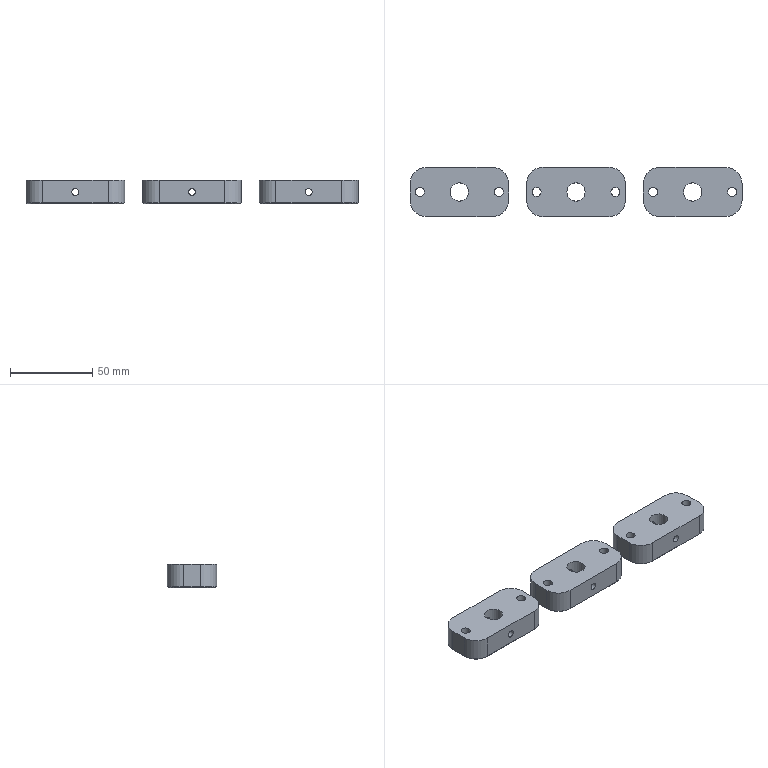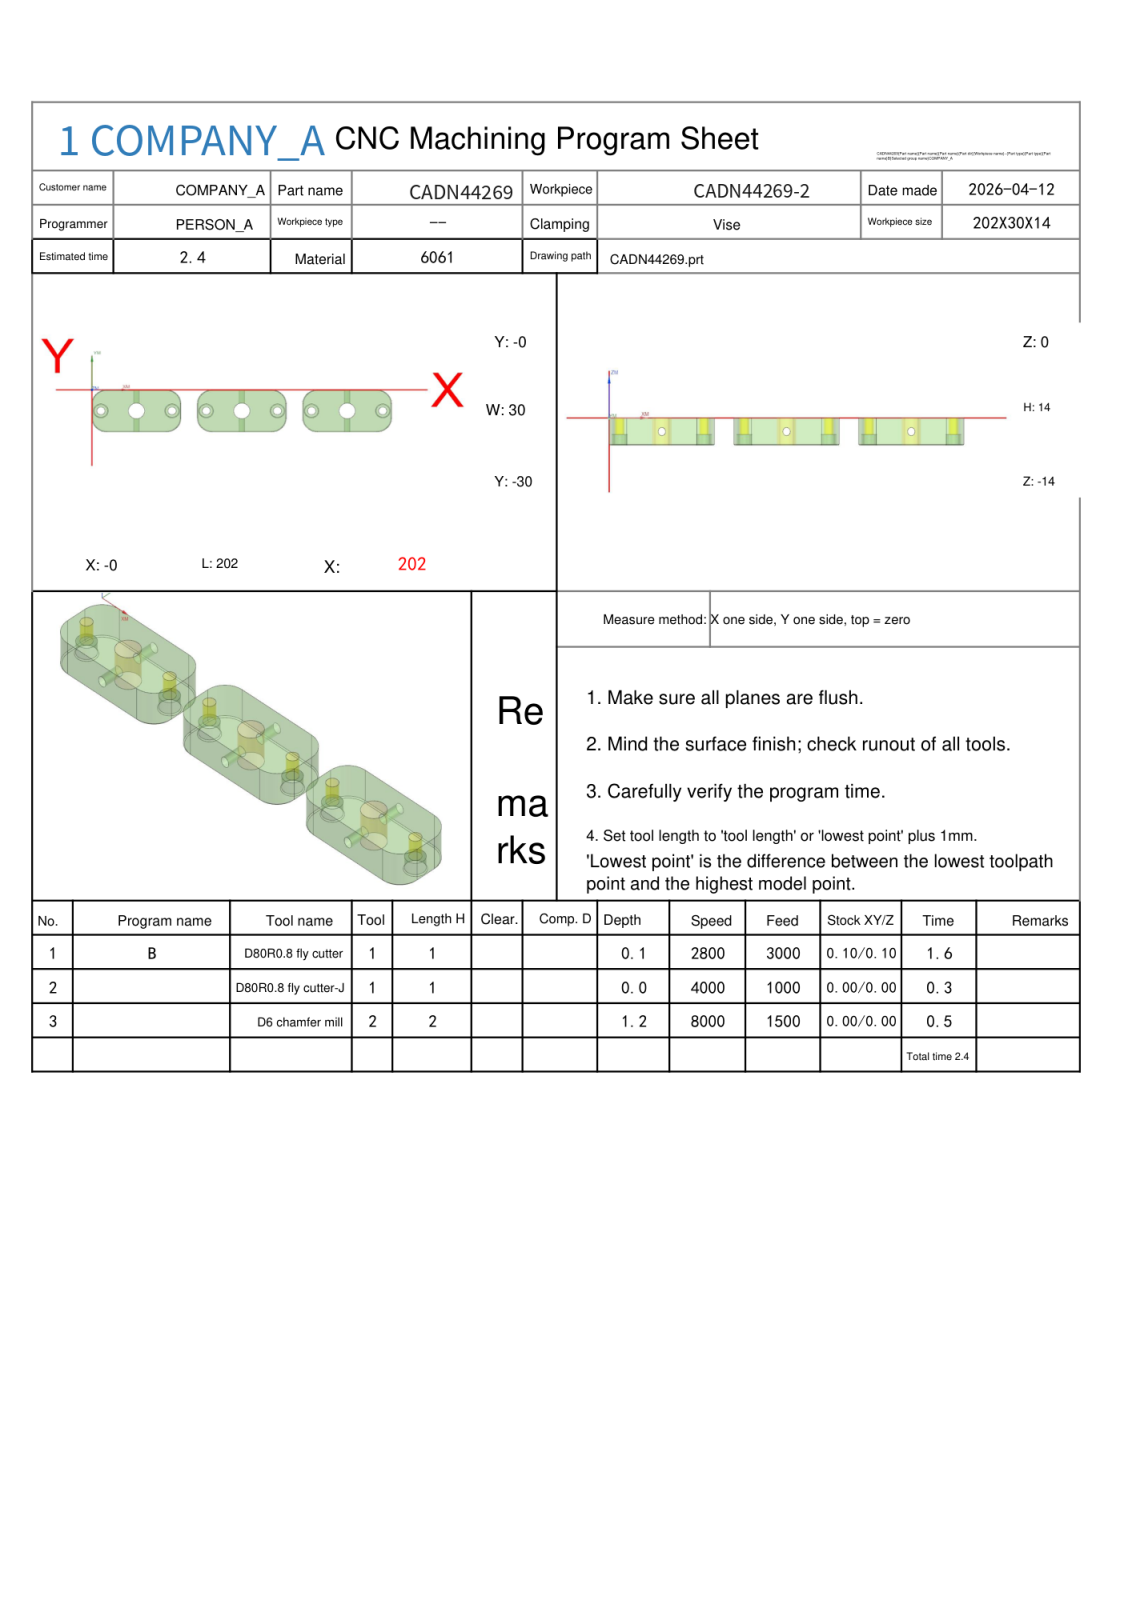NC program | NX | posted by the shop | part box 202 x 30 x 14 mm
Whole program:
%
O0001
(Machine time: 2.96 MIN)
(===Total Tool:2===)
(T1=D80R0.8 fly cutter D=80.  R=0.8  D-  H01 Z=0.    )
(T2=D6 chamfer mill   D=6.   R=0.   D-  H02 Z=-1.2  )
G80 G90 G17 G49 G40
G91 G28 Z0
M01
N1 T01 M06
(D80R0.8 fly cutter  D=80. R=0.8 H=01 ce=0.10 di=0.10)
G00 G90 G54 X-52.097 Y-15. M03 S2800
G43 H01 Z20.
M08
Z7.325
G01 Z5.325 F3000.
X-40.097
X242.097
X254.097
Z7.325
G00 X-52.097
Z6.85
G01 Z4.85
X-40.097
X242.097
X254.097
Z6.85
G00 X-52.097
Z6.375
G01 Z4.375
X-40.097
X242.097
X254.097
Z6.375
G00 X-52.097
Z5.9
G01 Z3.9
X-40.097
X242.097
X254.097
Z5.9
G00 Z20.
X-52.097
Z5.425
G01 Z3.425
X-40.097
X242.097
X254.097
Z5.425
G00 Z20.
X-52.097
Z4.95
G01 Z2.95
X-40.097
X242.097
X254.097
Z4.95
G00 Z20.
X-52.097
Z4.475
G01 Z2.475
X-40.097
X242.097
X254.097
Z4.475
G00 Z20.
X-52.097
Z4.
G01 Z2.
X-40.097
X242.097
X254.097
Z4.
G00 Z20.
X-52.097
Z3.525
G01 Z1.525
X-40.097
X242.097
X254.097
Z3.525
G00 Z20.
X-52.097
Z3.05
G01 Z1.05
X-40.097
X242.097
X254.097
Z3.05
G00 Z20.
X-52.097
Z2.575
G01 Z.575
X-40.097
X242.097
X254.097
Z2.575
G00 Z20.
X-52.097
Z2.1
G01 Z.1
X-40.097
X242.097
X254.097
Z2.1
G00 Z20.
G91 G28 Z0.0
M05
M09
G91 G28 Z0.0
M01
N2 T01 M06
(D80R0.8 fly cutter-J  D=80. R=0.8 H=01 ce=0.00 di=0.00)
G00 G90 G54 X-51.999 Y-15. M03 S4000
G43 H01 Z20.
M08
Z2.
G01 Z0.0 F1000.
X-39.999
X241.999
X253.999
Z2.
G00 Z20.
G91 G28 Z0.0
M05
M09
G91 G28 Z0.0
M01
N3 T02 M06
(D6 chamfer mill  D=6. R=0. H=02 ce=0.00 di=0.00)
G00 G90 G54 X29.614 Y1.127 M03 S8000
G43 H02 Z20.
M08
Z.272
G01 Z-1.199 F1350.
G03 X29.9 Y.927 I1.286 J1.532
G01 X29.946 Y.897
X30. Y.9
X50. F1500.
G02 X60.9 Y-10. I0.0 J-10.9
G01 Y-20.
G02 X50. Y-30.9 I-10.9 J0.0
G01 X10.
G02 X-.9 Y-20. I0.0 J10.9
G01 Y-10.
G02 X10. Y.9 I10.9 J0.0
G01 X30.
X30.054 Y.897
X30.1 Y.927
G03 X30.386 Y1.127 I-1. J1.732
G01 Z.272
G00 Z10.
X55.658 Y-15.404
Z.365
G01 Z-1.199 F1350.
G03 X55.832 Y-15.102 I-1.638 J1.147
G01 X55.858 Y-15.054
X55.85 Y-15.
G03 X54. Y-13.15 I-1.85 J0.0 F1500.
X52.15 Y-15. I0.0 J-1.85
X54. Y-16.85 I1.85 J0.0
X55.822 Y-15.321 I0.0 J1.85
G01 X55.85 Y-15.
X55.858 Y-14.946
X55.832 Y-14.898
G03 X55.658 Y-14.596 I-1.813 J-.845
G01 Z.365
G00 Z10.
X25.571 Y-14.6
Z.323
G01 Z-1.199 F1350.
G03 X25.39 Y-14.898 I1.613 J-1.183
G01 X25.364 Y-14.946
X25.37 Y-15.
G03 X30. Y-19.63 I4.63 J0.0 F1500.
X34.63 Y-15. I0.0 J4.63
X30. Y-10.37 I-4.63 J0.0
X25.37 Y-15. I0.0 J-4.63
G01 X25.364 Y-15.054
X25.39 Y-15.102
G03 X25.571 Y-15.4 I1.794 J.885
G01 Z.323
G00 Z10.
X7.658 Y-15.404
Z.365
G01 Z-1.199 F1350.
G03 X7.832 Y-15.102 I-1.638 J1.147
G01 X7.858 Y-15.054
X7.85 Y-15.
G03 X6. Y-13.15 I-1.85 J0.0 F1500.
X4.15 Y-15. I0.0 J-1.85
X6. Y-16.85 I1.85 J0.0
X7.822 Y-15.321 I0.0 J1.85
G01 X7.85 Y-15.
X7.858 Y-14.946
X7.832 Y-14.898
G03 X7.658 Y-14.596 I-1.813 J-.845
G01 Z.365
G00 Z10.
X100.614 Y1.127
Z.272
G01 Z-1.199 F1350.
G03 X100.9 Y.927 I1.286 J1.532
G01 X100.946 Y.897
X101. Y.9
X121. F1500.
G02 X131.9 Y-10. I0.0 J-10.9
G01 Y-20.
G02 X121. Y-30.9 I-10.9 J0.0
G01 X81.
G02 X70.1 Y-20. I0.0 J10.9
G01 Y-10.
G02 X81. Y.9 I10.9 J0.0
G01 X101.
X101.054 Y.897
X101.1 Y.927
G03 X101.386 Y1.127 I-1. J1.732
G01 Z.272
G00 Z10.
X126.658 Y-15.404
Z.365
G01 Z-1.199 F1350.
G03 X126.832 Y-15.102 I-1.638 J1.147
G01 X126.858 Y-15.054
X126.85 Y-15.
G03 X125. Y-13.15 I-1.85 J0.0 F1500.
X123.15 Y-15. I0.0 J-1.85
X125. Y-16.85 I1.85 J0.0
X126.822 Y-15.321 I0.0 J1.85
G01 X126.85 Y-15.
X126.858 Y-14.946
X126.832 Y-14.898
G03 X126.658 Y-14.596 I-1.813 J-.845
G01 Z.365
G00 Z10.
X96.571 Y-14.6
Z.323
G01 Z-1.199 F1350.
G03 X96.39 Y-14.898 I1.613 J-1.183
G01 X96.364 Y-14.946
X96.37 Y-15.
G03 X101. Y-19.63 I4.63 J0.0 F1500.
X105.63 Y-15. I0.0 J4.63
X101. Y-10.37 I-4.63 J0.0
X96.37 Y-15. I0.0 J-4.63
G01 X96.364 Y-15.054
X96.39 Y-15.102
G03 X96.571 Y-15.4 I1.794 J.885
G01 Z.323
G00 Z10.
X78.658 Y-15.404
Z.365
G01 Z-1.199 F1350.
G03 X78.832 Y-15.102 I-1.638 J1.147
G01 X78.858 Y-15.054
X78.85 Y-15.
G03 X77. Y-13.15 I-1.85 J0.0 F1500.
X75.15 Y-15. I0.0 J-1.85
X77. Y-16.85 I1.85 J0.0
X78.822 Y-15.321 I0.0 J1.85
G01 X78.85 Y-15.
X78.858 Y-14.946
X78.832 Y-14.898
G03 X78.658 Y-14.596 I-1.813 J-.845
G01 Z.365
G00 Z10.
X171.614 Y1.127
Z.272
G01 Z-1.199 F1350.
G03 X171.9 Y.927 I1.286 J1.532
G01 X171.946 Y.897
X172. Y.9
X192. F1500.
G02 X202.9 Y-10. I0.0 J-10.9
G01 Y-20.
G02 X192. Y-30.9 I-10.9 J0.0
G01 X152.
G02 X141.1 Y-20. I0.0 J10.9
G01 Y-10.
G02 X152. Y.9 I10.9 J0.0
G01 X172.
X172.054 Y.897
X172.1 Y.927
G03 X172.386 Y1.127 I-1. J1.732
G01 Z.272
G00 Z10.
X197.658 Y-15.404
Z.365
G01 Z-1.199 F1350.
G03 X197.832 Y-15.102 I-1.638 J1.147
G01 X197.858 Y-15.054
X197.85 Y-15.
G03 X196. Y-13.15 I-1.85 J0.0 F1500.
X194.15 Y-15. I0.0 J-1.85
X196. Y-16.85 I1.85 J0.0
X197.822 Y-15.321 I0.0 J1.85
G01 X197.85 Y-15.
X197.858 Y-14.946
X197.832 Y-14.898
G03 X197.658 Y-14.596 I-1.813 J-.845
G01 Z.365
G00 Z10.
X167.571 Y-14.6
Z.323
G01 Z-1.199 F1350.
G03 X167.39 Y-14.898 I1.613 J-1.183
G01 X167.364 Y-14.946
X167.37 Y-15.
G03 X172. Y-19.63 I4.63 J0.0 F1500.
X176.63 Y-15. I0.0 J4.63
X172. Y-10.37 I-4.63 J0.0
X167.37 Y-15. I0.0 J-4.63
G01 X167.364 Y-15.054
X167.39 Y-15.102
G03 X167.571 Y-15.4 I1.794 J.885
G01 Z.323
G00 Z10.
X149.658 Y-15.404
Z.365
G01 Z-1.199 F1350.
G03 X149.832 Y-15.102 I-1.638 J1.147
G01 X149.858 Y-15.054
X149.85 Y-15.
G03 X148. Y-13.15 I-1.85 J0.0 F1500.
X146.15 Y-15. I0.0 J-1.85
X148. Y-16.85 I1.85 J0.0
X149.822 Y-15.321 I0.0 J1.85
G01 X149.85 Y-15.
X149.858 Y-14.946
X149.832 Y-14.898
G03 X149.658 Y-14.596 I-1.813 J-.845
G01 Z.365
G00 Z20.
M05
M09
G91 G28 Z0.0
G91 G28 Y0.0
M30
%